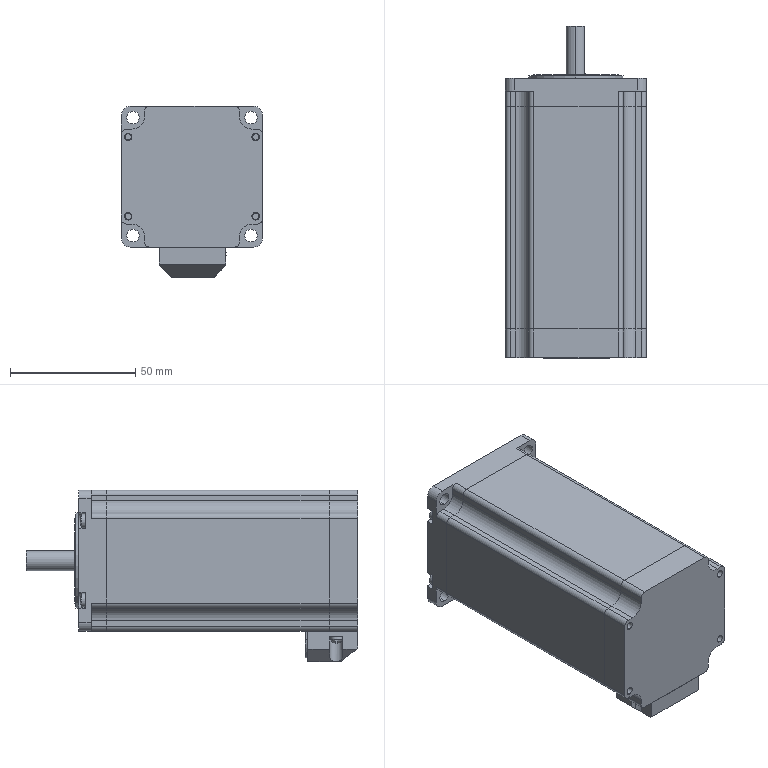Part | SolidWorks | features BaseBody 11 | 11 solids | 2572 faces | box 56.4 x 132.5 x 68.6 mm | volume 185240 mm3 | cone 1464 | cylinder 895 | plane 207 | sphere 6 | commonest cylinder face diameters 3 x760 4 x24 0.6 x16 37 x16 10 x14 5 x12